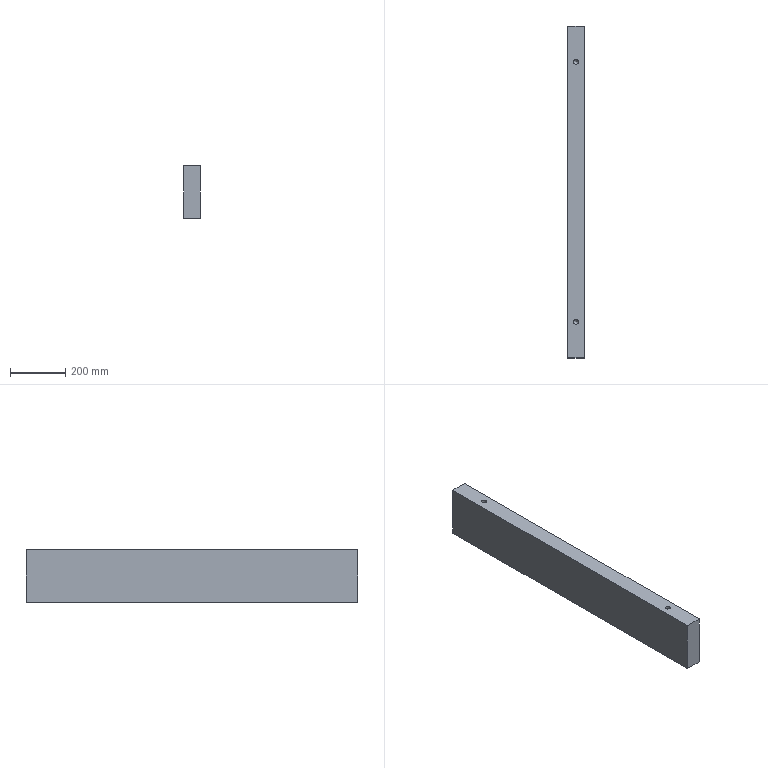Part | STEP file | lll_id4462_x_t | 1 solid | 14 faces | box 60 x 1200 x 190 mm | volume 13637476 mm3 | plane 6 | cylinder 4 | cone 4 | commonest cylinder face diameters 17.505 x2 17.506 x2
STEP:
#1=CARTESIAN_POINT('',(1247.435,-600.,-180.));
#2=VERTEX_POINT('',#1);
#3=CARTESIAN_POINT('',(1247.435,-600.,-370.));
#4=VERTEX_POINT('',#3);
#5=CARTESIAN_POINT('',(1247.435,-600.,-182.5));
#6=DIRECTION('',(0.,0.,-1.));
#7=VECTOR('',#6,1.);
#8=LINE('',#5,#7);
#9=EDGE_CURVE('',#2,#4,#8,.T.);
#10=ORIENTED_EDGE('',*,*,#9,.T.);
#11=CARTESIAN_POINT('',(1247.435,600.,-370.));
#12=VERTEX_POINT('',#11);
#13=CARTESIAN_POINT('',(1247.435,600.,-370.));
#14=DIRECTION('',(0.,-1.,0.));
#15=VECTOR('',#14,1.);
#16=LINE('',#13,#15);
#17=EDGE_CURVE('',#12,#4,#16,.T.);
#18=ORIENTED_EDGE('',*,*,#17,.F.);
#19=CARTESIAN_POINT('',(1247.435,600.,-180.));
#20=VERTEX_POINT('',#19);
#21=CARTESIAN_POINT('',(1247.435,600.,-182.5));
#22=DIRECTION('',(0.,0.,-1.));
#23=VECTOR('',#22,1.);
#24=LINE('',#21,#23);
#25=EDGE_CURVE('',#20,#12,#24,.T.);
#26=ORIENTED_EDGE('',*,*,#25,.F.);
#27=CARTESIAN_POINT('',(1247.435,1.,-180.));
#28=DIRECTION('',(0.,-1.,0.));
#29=VECTOR('',#28,1.);
#30=LINE('',#27,#29);
#31=EDGE_CURVE('',#20,#2,#30,.T.);
#32=ORIENTED_EDGE('',*,*,#31,.T.);
#33=EDGE_LOOP('',(#10,#18,#26,#32));
#34=FACE_OUTER_BOUND('',#33,.T.);
#35=CARTESIAN_POINT('',(1247.435,600.,-182.5));
#36=DIRECTION('',(1.,0.,0.));
#37=DIRECTION('',(0.,0.,-1.));
#38=AXIS2_PLACEMENT_3D('',#35,#36,#37);
#39=PLANE('',#38);
#40=ADVANCED_FACE('',(#34),#39,.T.);
#41=ORIENTED_EDGE('',*,*,#17,.T.);
#42=CARTESIAN_POINT('',(1187.435,-600.,-370.));
#43=VERTEX_POINT('',#42);
#44=CARTESIAN_POINT('',(1167.435,-600.,-370.));
#45=DIRECTION('',(-1.,0.,0.));
#46=VECTOR('',#45,1.);
#47=LINE('',#44,#46);
#48=EDGE_CURVE('',#4,#43,#47,.T.);
#49=ORIENTED_EDGE('',*,*,#48,.T.);
#50=CARTESIAN_POINT('',(1187.435,600.,-370.));
#51=VERTEX_POINT('',#50);
#52=CARTESIAN_POINT('',(1187.435,1.,-370.));
#53=DIRECTION('',(0.,-1.,0.));
#54=VECTOR('',#53,1.);
#55=LINE('',#52,#54);
#56=EDGE_CURVE('',#51,#43,#55,.T.);
#57=ORIENTED_EDGE('',*,*,#56,.F.);
#58=CARTESIAN_POINT('',(-2802.565,600.,-370.));
#59=DIRECTION('',(1.,0.,0.));
#60=VECTOR('',#59,1.);
#61=LINE('',#58,#60);
#62=EDGE_CURVE('',#51,#12,#61,.T.);
#63=ORIENTED_EDGE('',*,*,#62,.T.);
#64=EDGE_LOOP('',(#41,#49,#57,#63));
#65=FACE_BOUND('',#64,.T.);
#66=CARTESIAN_POINT('',(1226.188,-470.,-370.));
#67=VERTEX_POINT('',#66);
#68=CARTESIAN_POINT('',(1217.435,-470.,-370.));
#69=DIRECTION('',(0.,0.,1.));
#70=DIRECTION('',(1.,0.,0.));
#71=AXIS2_PLACEMENT_3D('',#68,#69,#70);
#72=CIRCLE('',#71,8.752);
#73=EDGE_CURVE('',#67,#67,#72,.T.);
#74=ORIENTED_EDGE('',*,*,#73,.T.);
#75=EDGE_LOOP('',(#74));
#76=FACE_BOUND('',#75,.T.);
#77=CARTESIAN_POINT('',(1226.188,470.,-370.));
#78=VERTEX_POINT('',#77);
#79=CARTESIAN_POINT('',(1217.435,470.,-370.));
#80=DIRECTION('',(0.,0.,1.));
#81=DIRECTION('',(1.,0.,0.));
#82=AXIS2_PLACEMENT_3D('',#79,#80,#81);
#83=CIRCLE('',#82,8.752);
#84=EDGE_CURVE('',#78,#78,#83,.T.);
#85=ORIENTED_EDGE('',*,*,#84,.T.);
#86=EDGE_LOOP('',(#85));
#87=FACE_BOUND('',#86,.T.);
#88=CARTESIAN_POINT('',(3433.751,1.,-370.));
#89=DIRECTION('',(0.,0.,-1.));
#90=DIRECTION('',(-1.,0.,0.));
#91=AXIS2_PLACEMENT_3D('',#88,#89,#90);
#92=PLANE('',#91);
#93=ADVANCED_FACE('',(#65,#76,#87),#92,.T.);
#94=CARTESIAN_POINT('',(1208.682,-470.,-180.));
#95=VERTEX_POINT('',#94);
#96=CARTESIAN_POINT('',(1217.435,-470.,-180.));
#97=DIRECTION('',(0.,0.,-1.));
#98=DIRECTION('',(-1.,0.,0.));
#99=AXIS2_PLACEMENT_3D('',#96,#97,#98);
#100=CIRCLE('',#99,8.753);
#101=EDGE_CURVE('',#95,#95,#100,.T.);
#102=ORIENTED_EDGE('',*,*,#101,.T.);
#103=EDGE_LOOP('',(#102));
#104=FACE_BOUND('',#103,.T.);
#105=CARTESIAN_POINT('',(1208.682,470.,-180.));
#106=VERTEX_POINT('',#105);
#107=CARTESIAN_POINT('',(1217.435,470.,-180.));
#108=DIRECTION('',(0.,0.,-1.));
#109=DIRECTION('',(-1.,0.,0.));
#110=AXIS2_PLACEMENT_3D('',#107,#108,#109);
#111=CIRCLE('',#110,8.753);
#112=EDGE_CURVE('',#106,#106,#111,.T.);
#113=ORIENTED_EDGE('',*,*,#112,.T.);
#114=EDGE_LOOP('',(#113));
#115=FACE_BOUND('',#114,.T.);
#116=CARTESIAN_POINT('',(1187.435,-600.,-180.));
#117=VERTEX_POINT('',#116);
#118=CARTESIAN_POINT('',(3353.751,-600.,-180.));
#119=DIRECTION('',(-1.,0.,0.));
#120=VECTOR('',#119,1.);
#121=LINE('',#118,#120);
#122=EDGE_CURVE('',#2,#117,#121,.T.);
#123=ORIENTED_EDGE('',*,*,#122,.F.);
#124=ORIENTED_EDGE('',*,*,#31,.F.);
#125=CARTESIAN_POINT('',(1187.435,600.,-180.));
#126=VERTEX_POINT('',#125);
#127=CARTESIAN_POINT('',(3353.751,600.,-180.));
#128=DIRECTION('',(1.,0.,0.));
#129=VECTOR('',#128,1.);
#130=LINE('',#127,#129);
#131=EDGE_CURVE('',#126,#20,#130,.T.);
#132=ORIENTED_EDGE('',*,*,#131,.F.);
#133=CARTESIAN_POINT('',(1187.435,0.,-180.));
#134=DIRECTION('',(0.,1.,0.));
#135=VECTOR('',#134,1.);
#136=LINE('',#133,#135);
#137=EDGE_CURVE('',#117,#126,#136,.T.);
#138=ORIENTED_EDGE('',*,*,#137,.F.);
#139=EDGE_LOOP('',(#123,#124,#132,#138));
#140=FACE_BOUND('',#139,.T.);
#141=CARTESIAN_POINT('',(3433.751,1.,-180.));
#142=DIRECTION('',(0.,0.,-1.));
#143=DIRECTION('',(-1.,0.,0.));
#144=AXIS2_PLACEMENT_3D('',#141,#142,#143);
#145=PLANE('',#144);
#146=ADVANCED_FACE('',(#104,#115,#140),#145,.F.);
#147=ORIENTED_EDGE('',*,*,#137,.T.);
#148=CARTESIAN_POINT('',(1187.435,600.,-251.25));
#149=DIRECTION('',(0.,0.,1.));
#150=VECTOR('',#149,1.);
#151=LINE('',#148,#150);
#152=EDGE_CURVE('',#51,#126,#151,.T.);
#153=ORIENTED_EDGE('',*,*,#152,.F.);
#154=ORIENTED_EDGE('',*,*,#56,.T.);
#155=CARTESIAN_POINT('',(1187.435,-600.,-251.25));
#156=DIRECTION('',(0.,0.,-1.));
#157=VECTOR('',#156,1.);
#158=LINE('',#155,#157);
#159=EDGE_CURVE('',#117,#43,#158,.T.);
#160=ORIENTED_EDGE('',*,*,#159,.F.);
#161=EDGE_LOOP('',(#147,#153,#154,#160));
#162=FACE_OUTER_BOUND('',#161,.T.);
#163=CARTESIAN_POINT('',(1187.435,0.,-251.25));
#164=DIRECTION('',(1.,0.,0.));
#165=DIRECTION('',(0.,0.,-1.));
#166=AXIS2_PLACEMENT_3D('',#163,#164,#165);
#167=PLANE('',#166);
#168=ADVANCED_FACE('',(#162),#167,.F.);
#169=ORIENTED_EDGE('',*,*,#159,.T.);
#170=ORIENTED_EDGE('',*,*,#48,.F.);
#171=ORIENTED_EDGE('',*,*,#9,.F.);
#172=ORIENTED_EDGE('',*,*,#122,.T.);
#173=EDGE_LOOP('',(#169,#170,#171,#172));
#174=FACE_OUTER_BOUND('',#173,.T.);
#175=CARTESIAN_POINT('',(1167.435,-600.,-182.5));
#176=DIRECTION('',(0.,-1.,0.));
#177=DIRECTION('',(0.,0.,-1.));
#178=AXIS2_PLACEMENT_3D('',#175,#176,#177);
#179=PLANE('',#178);
#180=ADVANCED_FACE('',(#174),#179,.T.);
#181=ORIENTED_EDGE('',*,*,#152,.T.);
#182=ORIENTED_EDGE('',*,*,#131,.T.);
#183=ORIENTED_EDGE('',*,*,#25,.T.);
#184=ORIENTED_EDGE('',*,*,#62,.F.);
#185=EDGE_LOOP('',(#181,#182,#183,#184));
#186=FACE_OUTER_BOUND('',#185,.T.);
#187=CARTESIAN_POINT('',(-2802.565,600.,-182.5));
#188=DIRECTION('',(0.,1.,0.));
#189=DIRECTION('',(0.,0.,1.));
#190=AXIS2_PLACEMENT_3D('',#187,#188,#189);
#191=PLANE('',#190);
#192=ADVANCED_FACE('',(#186),#191,.T.);
#193=CARTESIAN_POINT('',(1226.188,-470.,-328.747));
#194=VERTEX_POINT('',#193);
#195=CARTESIAN_POINT('',(1217.435,-470.,-328.747));
#196=DIRECTION('',(0.,0.,1.));
#197=DIRECTION('',(1.,0.,0.));
#198=AXIS2_PLACEMENT_3D('',#195,#196,#197);
#199=CIRCLE('',#198,8.752);
#200=EDGE_CURVE('',#194,#194,#199,.T.);
#201=ORIENTED_EDGE('',*,*,#200,.T.);
#202=EDGE_LOOP('',(#201));
#203=FACE_BOUND('',#202,.T.);
#204=ORIENTED_EDGE('',*,*,#73,.F.);
#205=EDGE_LOOP('',(#204));
#206=FACE_BOUND('',#205,.T.);
#207=CARTESIAN_POINT('',(1217.435,-470.,-370.));
#208=DIRECTION('',(0.,0.,1.));
#209=DIRECTION('',(-1.,0.,0.));
#210=AXIS2_PLACEMENT_3D('',#207,#208,#209);
#211=CYLINDRICAL_SURFACE('',#210,8.752);
#212=ADVANCED_FACE('',(#203,#206),#211,.F.);
#213=CARTESIAN_POINT('',(1217.435,-470.,-319.994));
#214=VERTEX_POINT('',#213);
#215=VERTEX_LOOP('',#214);
#216=FACE_BOUND('',#215,.T.);
#217=ORIENTED_EDGE('',*,*,#200,.F.);
#218=EDGE_LOOP('',(#217));
#219=FACE_BOUND('',#218,.T.);
#220=CARTESIAN_POINT('',(1217.435,-470.,-328.747));
#221=DIRECTION('',(0.,0.,-1.));
#222=DIRECTION('',(1.,0.,0.));
#223=AXIS2_PLACEMENT_3D('',#220,#221,#222);
#224=CONICAL_SURFACE('',#223,8.752,45.);
#225=ADVANCED_FACE('',(#216,#219),#224,.F.);
#226=CARTESIAN_POINT('',(1226.188,470.,-328.747));
#227=VERTEX_POINT('',#226);
#228=CARTESIAN_POINT('',(1217.435,470.,-328.747));
#229=DIRECTION('',(0.,0.,1.));
#230=DIRECTION('',(1.,0.,0.));
#231=AXIS2_PLACEMENT_3D('',#228,#229,#230);
#232=CIRCLE('',#231,8.752);
#233=EDGE_CURVE('',#227,#227,#232,.T.);
#234=ORIENTED_EDGE('',*,*,#233,.T.);
#235=EDGE_LOOP('',(#234));
#236=FACE_BOUND('',#235,.T.);
#237=ORIENTED_EDGE('',*,*,#84,.F.);
#238=EDGE_LOOP('',(#237));
#239=FACE_BOUND('',#238,.T.);
#240=CARTESIAN_POINT('',(1217.435,470.,-370.));
#241=DIRECTION('',(0.,0.,1.));
#242=DIRECTION('',(-1.,0.,0.));
#243=AXIS2_PLACEMENT_3D('',#240,#241,#242);
#244=CYLINDRICAL_SURFACE('',#243,8.752);
#245=ADVANCED_FACE('',(#236,#239),#244,.F.);
#246=CARTESIAN_POINT('',(1217.435,470.,-319.994));
#247=VERTEX_POINT('',#246);
#248=VERTEX_LOOP('',#247);
#249=FACE_BOUND('',#248,.T.);
#250=ORIENTED_EDGE('',*,*,#233,.F.);
#251=EDGE_LOOP('',(#250));
#252=FACE_BOUND('',#251,.T.);
#253=CARTESIAN_POINT('',(1217.435,470.,-328.747));
#254=DIRECTION('',(0.,0.,-1.));
#255=DIRECTION('',(1.,0.,0.));
#256=AXIS2_PLACEMENT_3D('',#253,#254,#255);
#257=CONICAL_SURFACE('',#256,8.752,45.);
#258=ADVANCED_FACE('',(#249,#252),#257,.F.);
#259=CARTESIAN_POINT('',(1208.682,470.,-221.253));
#260=VERTEX_POINT('',#259);
#261=CARTESIAN_POINT('',(1217.435,470.,-221.253));
#262=DIRECTION('',(0.,0.,-1.));
#263=DIRECTION('',(-1.,0.,0.));
#264=AXIS2_PLACEMENT_3D('',#261,#262,#263);
#265=CIRCLE('',#264,8.753);
#266=EDGE_CURVE('',#260,#260,#265,.T.);
#267=ORIENTED_EDGE('',*,*,#266,.T.);
#268=EDGE_LOOP('',(#267));
#269=FACE_BOUND('',#268,.T.);
#270=ORIENTED_EDGE('',*,*,#112,.F.);
#271=EDGE_LOOP('',(#270));
#272=FACE_BOUND('',#271,.T.);
#273=CARTESIAN_POINT('',(1217.435,470.,-180.));
#274=DIRECTION('',(0.,0.,-1.));
#275=DIRECTION('',(1.,0.,0.));
#276=AXIS2_PLACEMENT_3D('',#273,#274,#275);
#277=CYLINDRICAL_SURFACE('',#276,8.753);
#278=ADVANCED_FACE('',(#269,#272),#277,.F.);
#279=CARTESIAN_POINT('',(1217.435,470.,-230.006));
#280=VERTEX_POINT('',#279);
#281=VERTEX_LOOP('',#280);
#282=FACE_BOUND('',#281,.T.);
#283=ORIENTED_EDGE('',*,*,#266,.F.);
#284=EDGE_LOOP('',(#283));
#285=FACE_BOUND('',#284,.T.);
#286=CARTESIAN_POINT('',(1217.435,470.,-221.253));
#287=DIRECTION('',(0.,0.,1.));
#288=DIRECTION('',(-1.,0.,0.));
#289=AXIS2_PLACEMENT_3D('',#286,#287,#288);
#290=CONICAL_SURFACE('',#289,8.753,45.);
#291=ADVANCED_FACE('',(#282,#285),#290,.F.);
#292=CARTESIAN_POINT('',(1208.682,-470.,-221.253));
#293=VERTEX_POINT('',#292);
#294=CARTESIAN_POINT('',(1217.435,-470.,-221.253));
#295=DIRECTION('',(0.,0.,-1.));
#296=DIRECTION('',(-1.,0.,0.));
#297=AXIS2_PLACEMENT_3D('',#294,#295,#296);
#298=CIRCLE('',#297,8.753);
#299=EDGE_CURVE('',#293,#293,#298,.T.);
#300=ORIENTED_EDGE('',*,*,#299,.T.);
#301=EDGE_LOOP('',(#300));
#302=FACE_BOUND('',#301,.T.);
#303=ORIENTED_EDGE('',*,*,#101,.F.);
#304=EDGE_LOOP('',(#303));
#305=FACE_BOUND('',#304,.T.);
#306=CARTESIAN_POINT('',(1217.435,-470.,-180.));
#307=DIRECTION('',(0.,0.,-1.));
#308=DIRECTION('',(1.,0.,0.));
#309=AXIS2_PLACEMENT_3D('',#306,#307,#308);
#310=CYLINDRICAL_SURFACE('',#309,8.753);
#311=ADVANCED_FACE('',(#302,#305),#310,.F.);
#312=CARTESIAN_POINT('',(1217.435,-470.,-230.006));
#313=VERTEX_POINT('',#312);
#314=VERTEX_LOOP('',#313);
#315=FACE_BOUND('',#314,.T.);
#316=ORIENTED_EDGE('',*,*,#299,.F.);
#317=EDGE_LOOP('',(#316));
#318=FACE_BOUND('',#317,.T.);
#319=CARTESIAN_POINT('',(1217.435,-470.,-221.253));
#320=DIRECTION('',(0.,0.,1.));
#321=DIRECTION('',(-1.,0.,0.));
#322=AXIS2_PLACEMENT_3D('',#319,#320,#321);
#323=CONICAL_SURFACE('',#322,8.753,45.);
#324=ADVANCED_FACE('',(#315,#318),#323,.F.);
#325=CLOSED_SHELL('',(#40,#93,#146,#168,#180,#192,#212,#225,#245,#258,#278,#291,#311,#324));
#326=MANIFOLD_SOLID_BREP('',#325);
#327=(LENGTH_UNIT()NAMED_UNIT(*)SI_UNIT(.MILLI.,.METRE.));
#328=UNCERTAINTY_MEASURE_WITH_UNIT(LENGTH_MEASURE(0.00002),#327,'','');
#329=(NAMED_UNIT(*)PLANE_ANGLE_UNIT()SI_UNIT($,.RADIAN.));
#330=PLANE_ANGLE_MEASURE_WITH_UNIT(PLANE_ANGLE_MEASURE(0.01745),#329);
#331=DIMENSIONAL_EXPONENTS(0.,0.,0.,0.,0.,0.,0.);
#332=(CONVERSION_BASED_UNIT('DEGREE',#330)NAMED_UNIT(#331)PLANE_ANGLE_UNIT());
#333=(NAMED_UNIT(*)SI_UNIT($,.STERADIAN.)SOLID_ANGLE_UNIT());
#334=(GEOMETRIC_REPRESENTATION_CONTEXT(3)GLOBAL_UNCERTAINTY_ASSIGNED_CONTEXT((#328))GLOBAL_UNIT_ASSIGNED_CONTEXT((#327,#332,#333))REPRESENTATION_CONTEXT('',''));
#335=ADVANCED_BREP_SHAPE_REPRESENTATION('',(#326),#334);